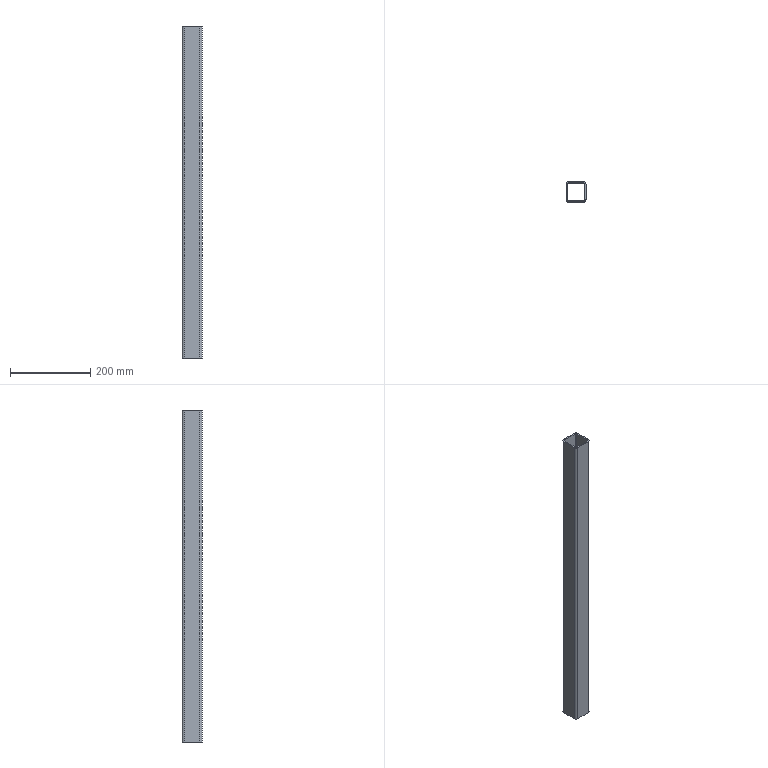Part | SolidWorks | 1 solid | 18 faces | box 50 x 50 x 830 mm | volume 448883 mm3 | plane 10 | cylinder 8 | commonest cylinder face diameters 6 x4 12 x4
STEP:
#1=CARTESIAN_POINT('',(19.,25.,415.));
#2=VERTEX_POINT('',#1);
#3=CARTESIAN_POINT('',(25.,19.,415.));
#4=VERTEX_POINT('',#3);
#5=CARTESIAN_POINT('',(19.,19.,415.));
#6=DIRECTION('',(0.,0.,-1.));
#7=DIRECTION('',(-1.,0.,0.));
#8=AXIS2_PLACEMENT_3D('',#5,#6,#7);
#9=CIRCLE('',#8,6.);
#10=EDGE_CURVE('',#2,#4,#9,.T.);
#11=ORIENTED_EDGE('',*,*,#10,.T.);
#12=CARTESIAN_POINT('',(25.,19.,-415.));
#13=VERTEX_POINT('',#12);
#14=CARTESIAN_POINT('',(25.,19.,-415.));
#15=DIRECTION('',(0.,0.,1.));
#16=VECTOR('',#15,1000.);
#17=LINE('',#14,#16);
#18=EDGE_CURVE('',#13,#4,#17,.T.);
#19=ORIENTED_EDGE('',*,*,#18,.F.);
#20=CARTESIAN_POINT('',(19.,25.,-415.));
#21=VERTEX_POINT('',#20);
#22=CARTESIAN_POINT('',(19.,19.,-415.));
#23=DIRECTION('',(0.,0.,-1.));
#24=DIRECTION('',(-1.,0.,0.));
#25=AXIS2_PLACEMENT_3D('',#22,#23,#24);
#26=CIRCLE('',#25,6.);
#27=EDGE_CURVE('',#21,#13,#26,.T.);
#28=ORIENTED_EDGE('',*,*,#27,.F.);
#29=CARTESIAN_POINT('',(19.,25.,-415.));
#30=DIRECTION('',(0.,0.,1.));
#31=VECTOR('',#30,1000.);
#32=LINE('',#29,#31);
#33=EDGE_CURVE('',#21,#2,#32,.T.);
#34=ORIENTED_EDGE('',*,*,#33,.T.);
#35=EDGE_LOOP('',(#11,#19,#28,#34));
#36=FACE_OUTER_BOUND('',#35,.T.);
#37=CARTESIAN_POINT('',(19.,19.,-415.));
#38=DIRECTION('',(0.,0.,1.));
#39=DIRECTION('',(1.,0.,0.));
#40=AXIS2_PLACEMENT_3D('',#37,#38,#39);
#41=CYLINDRICAL_SURFACE('',#40,6.);
#42=ADVANCED_FACE('',(#36),#41,.T.);
#43=CARTESIAN_POINT('',(25.,-19.,415.));
#44=VERTEX_POINT('',#43);
#45=CARTESIAN_POINT('',(25.,19.,415.));
#46=DIRECTION('',(0.,-1.,0.));
#47=VECTOR('',#46,1000.);
#48=LINE('',#45,#47);
#49=EDGE_CURVE('',#4,#44,#48,.T.);
#50=ORIENTED_EDGE('',*,*,#49,.T.);
#51=CARTESIAN_POINT('',(25.,-19.,-415.));
#52=VERTEX_POINT('',#51);
#53=CARTESIAN_POINT('',(25.,-19.,-415.));
#54=DIRECTION('',(0.,0.,1.));
#55=VECTOR('',#54,1000.);
#56=LINE('',#53,#55);
#57=EDGE_CURVE('',#52,#44,#56,.T.);
#58=ORIENTED_EDGE('',*,*,#57,.F.);
#59=CARTESIAN_POINT('',(25.,19.,-415.));
#60=DIRECTION('',(0.,-1.,0.));
#61=VECTOR('',#60,1000.);
#62=LINE('',#59,#61);
#63=EDGE_CURVE('',#13,#52,#62,.T.);
#64=ORIENTED_EDGE('',*,*,#63,.F.);
#65=ORIENTED_EDGE('',*,*,#18,.T.);
#66=EDGE_LOOP('',(#50,#58,#64,#65));
#67=FACE_OUTER_BOUND('',#66,.T.);
#68=CARTESIAN_POINT('',(25.,19.,-415.));
#69=DIRECTION('',(-1.,0.,0.));
#70=DIRECTION('',(0.,0.,1.));
#71=AXIS2_PLACEMENT_3D('',#68,#69,#70);
#72=PLANE('',#71);
#73=ADVANCED_FACE('',(#67),#72,.F.);
#74=CARTESIAN_POINT('',(19.,-25.,415.));
#75=VERTEX_POINT('',#74);
#76=CARTESIAN_POINT('',(19.,-19.,415.));
#77=DIRECTION('',(0.,0.,-1.));
#78=DIRECTION('',(-1.,0.,0.));
#79=AXIS2_PLACEMENT_3D('',#76,#77,#78);
#80=CIRCLE('',#79,6.);
#81=EDGE_CURVE('',#44,#75,#80,.T.);
#82=ORIENTED_EDGE('',*,*,#81,.T.);
#83=CARTESIAN_POINT('',(19.,-25.,-415.));
#84=VERTEX_POINT('',#83);
#85=CARTESIAN_POINT('',(19.,-25.,-415.));
#86=DIRECTION('',(0.,0.,1.));
#87=VECTOR('',#86,1000.);
#88=LINE('',#85,#87);
#89=EDGE_CURVE('',#84,#75,#88,.T.);
#90=ORIENTED_EDGE('',*,*,#89,.F.);
#91=CARTESIAN_POINT('',(19.,-19.,-415.));
#92=DIRECTION('',(0.,0.,-1.));
#93=DIRECTION('',(-1.,0.,0.));
#94=AXIS2_PLACEMENT_3D('',#91,#92,#93);
#95=CIRCLE('',#94,6.);
#96=EDGE_CURVE('',#52,#84,#95,.T.);
#97=ORIENTED_EDGE('',*,*,#96,.F.);
#98=ORIENTED_EDGE('',*,*,#57,.T.);
#99=EDGE_LOOP('',(#82,#90,#97,#98));
#100=FACE_OUTER_BOUND('',#99,.T.);
#101=CARTESIAN_POINT('',(19.,-19.,-415.));
#102=DIRECTION('',(0.,0.,1.));
#103=DIRECTION('',(1.,0.,0.));
#104=AXIS2_PLACEMENT_3D('',#101,#102,#103);
#105=CYLINDRICAL_SURFACE('',#104,6.);
#106=ADVANCED_FACE('',(#100),#105,.T.);
#107=CARTESIAN_POINT('',(-19.,-25.,415.));
#108=VERTEX_POINT('',#107);
#109=CARTESIAN_POINT('',(-19.,-25.,415.));
#110=DIRECTION('',(-1.,0.,0.));
#111=VECTOR('',#110,1000.);
#112=LINE('',#109,#111);
#113=EDGE_CURVE('',#75,#108,#112,.T.);
#114=ORIENTED_EDGE('',*,*,#113,.T.);
#115=CARTESIAN_POINT('',(-19.,-25.,-415.));
#116=VERTEX_POINT('',#115);
#117=CARTESIAN_POINT('',(-19.,-25.,-415.));
#118=DIRECTION('',(0.,0.,1.));
#119=VECTOR('',#118,1000.);
#120=LINE('',#117,#119);
#121=EDGE_CURVE('',#116,#108,#120,.T.);
#122=ORIENTED_EDGE('',*,*,#121,.F.);
#123=CARTESIAN_POINT('',(-19.,-25.,-415.));
#124=DIRECTION('',(-1.,0.,0.));
#125=VECTOR('',#124,1000.);
#126=LINE('',#123,#125);
#127=EDGE_CURVE('',#84,#116,#126,.T.);
#128=ORIENTED_EDGE('',*,*,#127,.F.);
#129=ORIENTED_EDGE('',*,*,#89,.T.);
#130=EDGE_LOOP('',(#114,#122,#128,#129));
#131=FACE_OUTER_BOUND('',#130,.T.);
#132=CARTESIAN_POINT('',(-19.,-25.,-415.));
#133=DIRECTION('',(0.,1.,0.));
#134=DIRECTION('',(0.,0.,1.));
#135=AXIS2_PLACEMENT_3D('',#132,#133,#134);
#136=PLANE('',#135);
#137=ADVANCED_FACE('',(#131),#136,.F.);
#138=CARTESIAN_POINT('',(-25.,-19.,415.));
#139=VERTEX_POINT('',#138);
#140=CARTESIAN_POINT('',(-19.,-19.,415.));
#141=DIRECTION('',(0.,0.,-1.));
#142=DIRECTION('',(-1.,0.,0.));
#143=AXIS2_PLACEMENT_3D('',#140,#141,#142);
#144=CIRCLE('',#143,6.);
#145=EDGE_CURVE('',#108,#139,#144,.T.);
#146=ORIENTED_EDGE('',*,*,#145,.T.);
#147=CARTESIAN_POINT('',(-25.,-19.,-415.));
#148=VERTEX_POINT('',#147);
#149=CARTESIAN_POINT('',(-25.,-19.,-415.));
#150=DIRECTION('',(0.,0.,1.));
#151=VECTOR('',#150,1000.);
#152=LINE('',#149,#151);
#153=EDGE_CURVE('',#148,#139,#152,.T.);
#154=ORIENTED_EDGE('',*,*,#153,.F.);
#155=CARTESIAN_POINT('',(-19.,-19.,-415.));
#156=DIRECTION('',(0.,0.,-1.));
#157=DIRECTION('',(-1.,0.,0.));
#158=AXIS2_PLACEMENT_3D('',#155,#156,#157);
#159=CIRCLE('',#158,6.);
#160=EDGE_CURVE('',#116,#148,#159,.T.);
#161=ORIENTED_EDGE('',*,*,#160,.F.);
#162=ORIENTED_EDGE('',*,*,#121,.T.);
#163=EDGE_LOOP('',(#146,#154,#161,#162));
#164=FACE_OUTER_BOUND('',#163,.T.);
#165=CARTESIAN_POINT('',(-19.,-19.,-415.));
#166=DIRECTION('',(0.,0.,1.));
#167=DIRECTION('',(1.,0.,0.));
#168=AXIS2_PLACEMENT_3D('',#165,#166,#167);
#169=CYLINDRICAL_SURFACE('',#168,6.);
#170=ADVANCED_FACE('',(#164),#169,.T.);
#171=CARTESIAN_POINT('',(-25.,19.,415.));
#172=VERTEX_POINT('',#171);
#173=CARTESIAN_POINT('',(-25.,-19.,415.));
#174=DIRECTION('',(0.,1.,0.));
#175=VECTOR('',#174,1000.);
#176=LINE('',#173,#175);
#177=EDGE_CURVE('',#139,#172,#176,.T.);
#178=ORIENTED_EDGE('',*,*,#177,.T.);
#179=CARTESIAN_POINT('',(-25.,19.,-415.));
#180=VERTEX_POINT('',#179);
#181=CARTESIAN_POINT('',(-25.,19.,-415.));
#182=DIRECTION('',(0.,0.,1.));
#183=VECTOR('',#182,1000.);
#184=LINE('',#181,#183);
#185=EDGE_CURVE('',#180,#172,#184,.T.);
#186=ORIENTED_EDGE('',*,*,#185,.F.);
#187=CARTESIAN_POINT('',(-25.,-19.,-415.));
#188=DIRECTION('',(0.,1.,0.));
#189=VECTOR('',#188,1000.);
#190=LINE('',#187,#189);
#191=EDGE_CURVE('',#148,#180,#190,.T.);
#192=ORIENTED_EDGE('',*,*,#191,.F.);
#193=ORIENTED_EDGE('',*,*,#153,.T.);
#194=EDGE_LOOP('',(#178,#186,#192,#193));
#195=FACE_OUTER_BOUND('',#194,.T.);
#196=CARTESIAN_POINT('',(-25.,-19.,-415.));
#197=DIRECTION('',(1.,0.,0.));
#198=DIRECTION('',(0.,0.,-1.));
#199=AXIS2_PLACEMENT_3D('',#196,#197,#198);
#200=PLANE('',#199);
#201=ADVANCED_FACE('',(#195),#200,.F.);
#202=CARTESIAN_POINT('',(-19.,25.,415.));
#203=VERTEX_POINT('',#202);
#204=CARTESIAN_POINT('',(-19.,19.,415.));
#205=DIRECTION('',(0.,0.,-1.));
#206=DIRECTION('',(-1.,0.,0.));
#207=AXIS2_PLACEMENT_3D('',#204,#205,#206);
#208=CIRCLE('',#207,6.);
#209=EDGE_CURVE('',#172,#203,#208,.T.);
#210=ORIENTED_EDGE('',*,*,#209,.T.);
#211=CARTESIAN_POINT('',(-19.,25.,-415.));
#212=VERTEX_POINT('',#211);
#213=CARTESIAN_POINT('',(-19.,25.,-415.));
#214=DIRECTION('',(0.,0.,1.));
#215=VECTOR('',#214,1000.);
#216=LINE('',#213,#215);
#217=EDGE_CURVE('',#212,#203,#216,.T.);
#218=ORIENTED_EDGE('',*,*,#217,.F.);
#219=CARTESIAN_POINT('',(-19.,19.,-415.));
#220=DIRECTION('',(0.,0.,-1.));
#221=DIRECTION('',(-1.,0.,0.));
#222=AXIS2_PLACEMENT_3D('',#219,#220,#221);
#223=CIRCLE('',#222,6.);
#224=EDGE_CURVE('',#180,#212,#223,.T.);
#225=ORIENTED_EDGE('',*,*,#224,.F.);
#226=ORIENTED_EDGE('',*,*,#185,.T.);
#227=EDGE_LOOP('',(#210,#218,#225,#226));
#228=FACE_OUTER_BOUND('',#227,.T.);
#229=CARTESIAN_POINT('',(-19.,19.,-415.));
#230=DIRECTION('',(0.,0.,1.));
#231=DIRECTION('',(1.,0.,0.));
#232=AXIS2_PLACEMENT_3D('',#229,#230,#231);
#233=CYLINDRICAL_SURFACE('',#232,6.);
#234=ADVANCED_FACE('',(#228),#233,.T.);
#235=CARTESIAN_POINT('',(22.,-19.,415.));
#236=VERTEX_POINT('',#235);
#237=CARTESIAN_POINT('',(19.,-22.,415.));
#238=VERTEX_POINT('',#237);
#239=CARTESIAN_POINT('',(19.,-19.,415.));
#240=DIRECTION('',(0.,0.,-1.));
#241=DIRECTION('',(-1.,0.,0.));
#242=AXIS2_PLACEMENT_3D('',#239,#240,#241);
#243=CIRCLE('',#242,3.);
#244=EDGE_CURVE('',#236,#238,#243,.T.);
#245=ORIENTED_EDGE('',*,*,#244,.F.);
#246=CARTESIAN_POINT('',(22.,-19.,-415.));
#247=VERTEX_POINT('',#246);
#248=CARTESIAN_POINT('',(22.,-19.,-415.));
#249=DIRECTION('',(0.,0.,1.));
#250=VECTOR('',#249,1000.);
#251=LINE('',#248,#250);
#252=EDGE_CURVE('',#247,#236,#251,.T.);
#253=ORIENTED_EDGE('',*,*,#252,.F.);
#254=CARTESIAN_POINT('',(19.,-22.,-415.));
#255=VERTEX_POINT('',#254);
#256=CARTESIAN_POINT('',(19.,-19.,-415.));
#257=DIRECTION('',(0.,0.,-1.));
#258=DIRECTION('',(-1.,0.,0.));
#259=AXIS2_PLACEMENT_3D('',#256,#257,#258);
#260=CIRCLE('',#259,3.);
#261=EDGE_CURVE('',#247,#255,#260,.T.);
#262=ORIENTED_EDGE('',*,*,#261,.T.);
#263=CARTESIAN_POINT('',(19.,-22.,-415.));
#264=DIRECTION('',(0.,0.,1.));
#265=VECTOR('',#264,1000.);
#266=LINE('',#263,#265);
#267=EDGE_CURVE('',#255,#238,#266,.T.);
#268=ORIENTED_EDGE('',*,*,#267,.T.);
#269=EDGE_LOOP('',(#245,#253,#262,#268));
#270=FACE_OUTER_BOUND('',#269,.T.);
#271=CARTESIAN_POINT('',(19.,-19.,-415.));
#272=DIRECTION('',(0.,0.,1.));
#273=DIRECTION('',(1.,0.,0.));
#274=AXIS2_PLACEMENT_3D('',#271,#272,#273);
#275=CYLINDRICAL_SURFACE('',#274,3.);
#276=ADVANCED_FACE('',(#270),#275,.F.);
#277=CARTESIAN_POINT('',(22.,19.,415.));
#278=VERTEX_POINT('',#277);
#279=CARTESIAN_POINT('',(22.,19.,415.));
#280=DIRECTION('',(0.,-1.,0.));
#281=VECTOR('',#280,1000.);
#282=LINE('',#279,#281);
#283=EDGE_CURVE('',#278,#236,#282,.T.);
#284=ORIENTED_EDGE('',*,*,#283,.F.);
#285=CARTESIAN_POINT('',(22.,19.,-415.));
#286=VERTEX_POINT('',#285);
#287=CARTESIAN_POINT('',(22.,19.,-415.));
#288=DIRECTION('',(0.,0.,1.));
#289=VECTOR('',#288,1000.);
#290=LINE('',#287,#289);
#291=EDGE_CURVE('',#286,#278,#290,.T.);
#292=ORIENTED_EDGE('',*,*,#291,.F.);
#293=CARTESIAN_POINT('',(22.,19.,-415.));
#294=DIRECTION('',(0.,-1.,0.));
#295=VECTOR('',#294,1000.);
#296=LINE('',#293,#295);
#297=EDGE_CURVE('',#286,#247,#296,.T.);
#298=ORIENTED_EDGE('',*,*,#297,.T.);
#299=ORIENTED_EDGE('',*,*,#252,.T.);
#300=EDGE_LOOP('',(#284,#292,#298,#299));
#301=FACE_OUTER_BOUND('',#300,.T.);
#302=CARTESIAN_POINT('',(22.,19.,-415.));
#303=DIRECTION('',(-1.,0.,0.));
#304=DIRECTION('',(0.,0.,1.));
#305=AXIS2_PLACEMENT_3D('',#302,#303,#304);
#306=PLANE('',#305);
#307=ADVANCED_FACE('',(#301),#306,.T.);
#308=CARTESIAN_POINT('',(19.,22.,415.));
#309=VERTEX_POINT('',#308);
#310=CARTESIAN_POINT('',(19.,19.,415.));
#311=DIRECTION('',(0.,0.,-1.));
#312=DIRECTION('',(-1.,0.,0.));
#313=AXIS2_PLACEMENT_3D('',#310,#311,#312);
#314=CIRCLE('',#313,3.);
#315=EDGE_CURVE('',#309,#278,#314,.T.);
#316=ORIENTED_EDGE('',*,*,#315,.F.);
#317=CARTESIAN_POINT('',(19.,22.,-415.));
#318=VERTEX_POINT('',#317);
#319=CARTESIAN_POINT('',(19.,22.,-415.));
#320=DIRECTION('',(0.,0.,1.));
#321=VECTOR('',#320,1000.);
#322=LINE('',#319,#321);
#323=EDGE_CURVE('',#318,#309,#322,.T.);
#324=ORIENTED_EDGE('',*,*,#323,.F.);
#325=CARTESIAN_POINT('',(19.,19.,-415.));
#326=DIRECTION('',(0.,0.,-1.));
#327=DIRECTION('',(-1.,0.,0.));
#328=AXIS2_PLACEMENT_3D('',#325,#326,#327);
#329=CIRCLE('',#328,3.);
#330=EDGE_CURVE('',#318,#286,#329,.T.);
#331=ORIENTED_EDGE('',*,*,#330,.T.);
#332=ORIENTED_EDGE('',*,*,#291,.T.);
#333=EDGE_LOOP('',(#316,#324,#331,#332));
#334=FACE_OUTER_BOUND('',#333,.T.);
#335=CARTESIAN_POINT('',(19.,19.,-415.));
#336=DIRECTION('',(0.,0.,1.));
#337=DIRECTION('',(1.,0.,0.));
#338=AXIS2_PLACEMENT_3D('',#335,#336,#337);
#339=CYLINDRICAL_SURFACE('',#338,3.);
#340=ADVANCED_FACE('',(#334),#339,.F.);
#341=CARTESIAN_POINT('',(-19.,22.,415.));
#342=VERTEX_POINT('',#341);
#343=CARTESIAN_POINT('',(19.,22.,415.));
#344=DIRECTION('',(1.,0.,0.));
#345=VECTOR('',#344,1000.);
#346=LINE('',#343,#345);
#347=EDGE_CURVE('',#342,#309,#346,.T.);
#348=ORIENTED_EDGE('',*,*,#347,.F.);
#349=CARTESIAN_POINT('',(-19.,22.,-415.));
#350=VERTEX_POINT('',#349);
#351=CARTESIAN_POINT('',(-19.,22.,-415.));
#352=DIRECTION('',(0.,0.,1.));
#353=VECTOR('',#352,1000.);
#354=LINE('',#351,#353);
#355=EDGE_CURVE('',#350,#342,#354,.T.);
#356=ORIENTED_EDGE('',*,*,#355,.F.);
#357=CARTESIAN_POINT('',(19.,22.,-415.));
#358=DIRECTION('',(1.,0.,0.));
#359=VECTOR('',#358,1000.);
#360=LINE('',#357,#359);
#361=EDGE_CURVE('',#350,#318,#360,.T.);
#362=ORIENTED_EDGE('',*,*,#361,.T.);
#363=ORIENTED_EDGE('',*,*,#323,.T.);
#364=EDGE_LOOP('',(#348,#356,#362,#363));
#365=FACE_OUTER_BOUND('',#364,.T.);
#366=CARTESIAN_POINT('',(19.,22.,-415.));
#367=DIRECTION('',(0.,-1.,0.));
#368=DIRECTION('',(0.,0.,-1.));
#369=AXIS2_PLACEMENT_3D('',#366,#367,#368);
#370=PLANE('',#369);
#371=ADVANCED_FACE('',(#365),#370,.T.);
#372=CARTESIAN_POINT('',(-22.,19.,415.));
#373=VERTEX_POINT('',#372);
#374=CARTESIAN_POINT('',(-19.,19.,415.));
#375=DIRECTION('',(0.,0.,-1.));
#376=DIRECTION('',(-1.,0.,0.));
#377=AXIS2_PLACEMENT_3D('',#374,#375,#376);
#378=CIRCLE('',#377,3.);
#379=EDGE_CURVE('',#373,#342,#378,.T.);
#380=ORIENTED_EDGE('',*,*,#379,.F.);
#381=CARTESIAN_POINT('',(-22.,19.,-415.));
#382=VERTEX_POINT('',#381);
#383=CARTESIAN_POINT('',(-22.,19.,-415.));
#384=DIRECTION('',(0.,0.,1.));
#385=VECTOR('',#384,1000.);
#386=LINE('',#383,#385);
#387=EDGE_CURVE('',#382,#373,#386,.T.);
#388=ORIENTED_EDGE('',*,*,#387,.F.);
#389=CARTESIAN_POINT('',(-19.,19.,-415.));
#390=DIRECTION('',(0.,0.,-1.));
#391=DIRECTION('',(-1.,0.,0.));
#392=AXIS2_PLACEMENT_3D('',#389,#390,#391);
#393=CIRCLE('',#392,3.);
#394=EDGE_CURVE('',#382,#350,#393,.T.);
#395=ORIENTED_EDGE('',*,*,#394,.T.);
#396=ORIENTED_EDGE('',*,*,#355,.T.);
#397=EDGE_LOOP('',(#380,#388,#395,#396));
#398=FACE_OUTER_BOUND('',#397,.T.);
#399=CARTESIAN_POINT('',(-19.,19.,-415.));
#400=DIRECTION('',(0.,0.,1.));
#401=DIRECTION('',(1.,0.,0.));
#402=AXIS2_PLACEMENT_3D('',#399,#400,#401);
#403=CYLINDRICAL_SURFACE('',#402,3.);
#404=ADVANCED_FACE('',(#398),#403,.F.);
#405=CARTESIAN_POINT('',(-22.,-19.,415.));
#406=VERTEX_POINT('',#405);
#407=CARTESIAN_POINT('',(-22.,-19.,415.));
#408=DIRECTION('',(0.,1.,0.));
#409=VECTOR('',#408,1000.);
#410=LINE('',#407,#409);
#411=EDGE_CURVE('',#406,#373,#410,.T.);
#412=ORIENTED_EDGE('',*,*,#411,.F.);
#413=CARTESIAN_POINT('',(-22.,-19.,-415.));
#414=VERTEX_POINT('',#413);
#415=CARTESIAN_POINT('',(-22.,-19.,-415.));
#416=DIRECTION('',(0.,0.,1.));
#417=VECTOR('',#416,1000.);
#418=LINE('',#415,#417);
#419=EDGE_CURVE('',#414,#406,#418,.T.);
#420=ORIENTED_EDGE('',*,*,#419,.F.);
#421=CARTESIAN_POINT('',(-22.,-19.,-415.));
#422=DIRECTION('',(0.,1.,0.));
#423=VECTOR('',#422,1000.);
#424=LINE('',#421,#423);
#425=EDGE_CURVE('',#414,#382,#424,.T.);
#426=ORIENTED_EDGE('',*,*,#425,.T.);
#427=ORIENTED_EDGE('',*,*,#387,.T.);
#428=EDGE_LOOP('',(#412,#420,#426,#427));
#429=FACE_OUTER_BOUND('',#428,.T.);
#430=CARTESIAN_POINT('',(-22.,-19.,-415.));
#431=DIRECTION('',(1.,0.,0.));
#432=DIRECTION('',(0.,0.,-1.));
#433=AXIS2_PLACEMENT_3D('',#430,#431,#432);
#434=PLANE('',#433);
#435=ADVANCED_FACE('',(#429),#434,.T.);
#436=CARTESIAN_POINT('',(-19.,-22.,415.));
#437=VERTEX_POINT('',#436);
#438=CARTESIAN_POINT('',(-19.,-19.,415.));
#439=DIRECTION('',(0.,0.,-1.));
#440=DIRECTION('',(-1.,0.,0.));
#441=AXIS2_PLACEMENT_3D('',#438,#439,#440);
#442=CIRCLE('',#441,3.);
#443=EDGE_CURVE('',#437,#406,#442,.T.);
#444=ORIENTED_EDGE('',*,*,#443,.F.);
#445=CARTESIAN_POINT('',(-19.,-22.,-415.));
#446=VERTEX_POINT('',#445);
#447=CARTESIAN_POINT('',(-19.,-22.,-415.));
#448=DIRECTION('',(0.,0.,1.));
#449=VECTOR('',#448,1000.);
#450=LINE('',#447,#449);
#451=EDGE_CURVE('',#446,#437,#450,.T.);
#452=ORIENTED_EDGE('',*,*,#451,.F.);
#453=CARTESIAN_POINT('',(-19.,-19.,-415.));
#454=DIRECTION('',(0.,0.,-1.));
#455=DIRECTION('',(-1.,0.,0.));
#456=AXIS2_PLACEMENT_3D('',#453,#454,#455);
#457=CIRCLE('',#456,3.);
#458=EDGE_CURVE('',#446,#414,#457,.T.);
#459=ORIENTED_EDGE('',*,*,#458,.T.);
#460=ORIENTED_EDGE('',*,*,#419,.T.);
#461=EDGE_LOOP('',(#444,#452,#459,#460));
#462=FACE_OUTER_BOUND('',#461,.T.);
#463=CARTESIAN_POINT('',(-19.,-19.,-415.));
#464=DIRECTION('',(0.,0.,1.));
#465=DIRECTION('',(1.,0.,0.));
#466=AXIS2_PLACEMENT_3D('',#463,#464,#465);
#467=CYLINDRICAL_SURFACE('',#466,3.);
#468=ADVANCED_FACE('',(#462),#467,.F.);
#469=CARTESIAN_POINT('',(-19.,-22.,415.));
#470=DIRECTION('',(-1.,0.,0.));
#471=VECTOR('',#470,1000.);
#472=LINE('',#469,#471);
#473=EDGE_CURVE('',#238,#437,#472,.T.);
#474=ORIENTED_EDGE('',*,*,#473,.F.);
#475=ORIENTED_EDGE('',*,*,#267,.F.);
#476=CARTESIAN_POINT('',(-19.,-22.,-415.));
#477=DIRECTION('',(-1.,0.,0.));
#478=VECTOR('',#477,1000.);
#479=LINE('',#476,#478);
#480=EDGE_CURVE('',#255,#446,#479,.T.);
#481=ORIENTED_EDGE('',*,*,#480,.T.);
#482=ORIENTED_EDGE('',*,*,#451,.T.);
#483=EDGE_LOOP('',(#474,#475,#481,#482));
#484=FACE_OUTER_BOUND('',#483,.T.);
#485=CARTESIAN_POINT('',(-19.,-22.,-415.));
#486=DIRECTION('',(0.,1.,0.));
#487=DIRECTION('',(0.,0.,1.));
#488=AXIS2_PLACEMENT_3D('',#485,#486,#487);
#489=PLANE('',#488);
#490=ADVANCED_FACE('',(#484),#489,.T.);
#491=CARTESIAN_POINT('',(19.,25.,415.));
#492=DIRECTION('',(1.,0.,0.));
#493=VECTOR('',#492,1000.);
#494=LINE('',#491,#493);
#495=EDGE_CURVE('',#203,#2,#494,.T.);
#496=ORIENTED_EDGE('',*,*,#495,.T.);
#497=ORIENTED_EDGE('',*,*,#33,.F.);
#498=CARTESIAN_POINT('',(19.,25.,-415.));
#499=DIRECTION('',(1.,0.,0.));
#500=VECTOR('',#499,1000.);
#501=LINE('',#498,#500);
#502=EDGE_CURVE('',#212,#21,#501,.T.);
#503=ORIENTED_EDGE('',*,*,#502,.F.);
#504=ORIENTED_EDGE('',*,*,#217,.T.);
#505=EDGE_LOOP('',(#496,#497,#503,#504));
#506=FACE_OUTER_BOUND('',#505,.T.);
#507=CARTESIAN_POINT('',(19.,25.,-415.));
#508=DIRECTION('',(0.,-1.,0.));
#509=DIRECTION('',(0.,0.,-1.));
#510=AXIS2_PLACEMENT_3D('',#507,#508,#509);
#511=PLANE('',#510);
#512=ADVANCED_FACE('',(#506),#511,.F.);
#513=ORIENTED_EDGE('',*,*,#261,.F.);
#514=ORIENTED_EDGE('',*,*,#297,.F.);
#515=ORIENTED_EDGE('',*,*,#330,.F.);
#516=ORIENTED_EDGE('',*,*,#361,.F.);
#517=ORIENTED_EDGE('',*,*,#394,.F.);
#518=ORIENTED_EDGE('',*,*,#425,.F.);
#519=ORIENTED_EDGE('',*,*,#458,.F.);
#520=ORIENTED_EDGE('',*,*,#480,.F.);
#521=EDGE_LOOP('',(#513,#514,#515,#516,#517,#518,#519,#520));
#522=FACE_BOUND('',#521,.T.);
#523=ORIENTED_EDGE('',*,*,#27,.T.);
#524=ORIENTED_EDGE('',*,*,#63,.T.);
#525=ORIENTED_EDGE('',*,*,#96,.T.);
#526=ORIENTED_EDGE('',*,*,#127,.T.);
#527=ORIENTED_EDGE('',*,*,#160,.T.);
#528=ORIENTED_EDGE('',*,*,#191,.T.);
#529=ORIENTED_EDGE('',*,*,#224,.T.);
#530=ORIENTED_EDGE('',*,*,#502,.T.);
#531=EDGE_LOOP('',(#523,#524,#525,#526,#527,#528,#529,#530));
#532=FACE_OUTER_BOUND('',#531,.T.);
#533=CARTESIAN_POINT('',(19.,19.,-415.));
#534=DIRECTION('',(0.,0.,-1.));
#535=DIRECTION('',(-1.,0.,0.));
#536=AXIS2_PLACEMENT_3D('',#533,#534,#535);
#537=PLANE('',#536);
#538=ADVANCED_FACE('',(#522,#532),#537,.T.);
#539=ORIENTED_EDGE('',*,*,#244,.T.);
#540=ORIENTED_EDGE('',*,*,#473,.T.);
#541=ORIENTED_EDGE('',*,*,#443,.T.);
#542=ORIENTED_EDGE('',*,*,#411,.T.);
#543=ORIENTED_EDGE('',*,*,#379,.T.);
#544=ORIENTED_EDGE('',*,*,#347,.T.);
#545=ORIENTED_EDGE('',*,*,#315,.T.);
#546=ORIENTED_EDGE('',*,*,#283,.T.);
#547=EDGE_LOOP('',(#539,#540,#541,#542,#543,#544,#545,#546));
#548=FACE_BOUND('',#547,.T.);
#549=ORIENTED_EDGE('',*,*,#10,.F.);
#550=ORIENTED_EDGE('',*,*,#495,.F.);
#551=ORIENTED_EDGE('',*,*,#209,.F.);
#552=ORIENTED_EDGE('',*,*,#177,.F.);
#553=ORIENTED_EDGE('',*,*,#145,.F.);
#554=ORIENTED_EDGE('',*,*,#113,.F.);
#555=ORIENTED_EDGE('',*,*,#81,.F.);
#556=ORIENTED_EDGE('',*,*,#49,.F.);
#557=EDGE_LOOP('',(#549,#550,#551,#552,#553,#554,#555,#556));
#558=FACE_OUTER_BOUND('',#557,.T.);
#559=CARTESIAN_POINT('',(19.,19.,415.));
#560=DIRECTION('',(0.,0.,-1.));
#561=DIRECTION('',(-1.,0.,0.));
#562=AXIS2_PLACEMENT_3D('',#559,#560,#561);
#563=PLANE('',#562);
#564=ADVANCED_FACE('',(#548,#558),#563,.F.);
#565=CLOSED_SHELL('',(#42,#73,#106,#137,#170,#201,#234,#276,#307,#340,#371,#404,#435,#468,#490,#512,#538,#564));
#566=MANIFOLD_SOLID_BREP('',#565);
#567=CARTESIAN_POINT('',(0.,0.,0.));
#568=DIRECTION('',(0.,0.,1.));
#569=DIRECTION('',(1.,0.,0.));
#570=AXIS2_PLACEMENT_3D('',#567,#568,#569);
#571=(LENGTH_UNIT()NAMED_UNIT(*)SI_UNIT(.MILLI.,.METRE.));
#572=UNCERTAINTY_MEASURE_WITH_UNIT(LENGTH_MEASURE(0.00001),#571,'','');
#573=(NAMED_UNIT(*)PLANE_ANGLE_UNIT()SI_UNIT($,.RADIAN.));
#574=(NAMED_UNIT(*)SI_UNIT($,.STERADIAN.)SOLID_ANGLE_UNIT());
#575=(GEOMETRIC_REPRESENTATION_CONTEXT(3)GLOBAL_UNCERTAINTY_ASSIGNED_CONTEXT((#572))GLOBAL_UNIT_ASSIGNED_CONTEXT((#571,#573,#574))REPRESENTATION_CONTEXT('',''));
#576=ADVANCED_BREP_SHAPE_REPRESENTATION('',(#566,#570),#575);